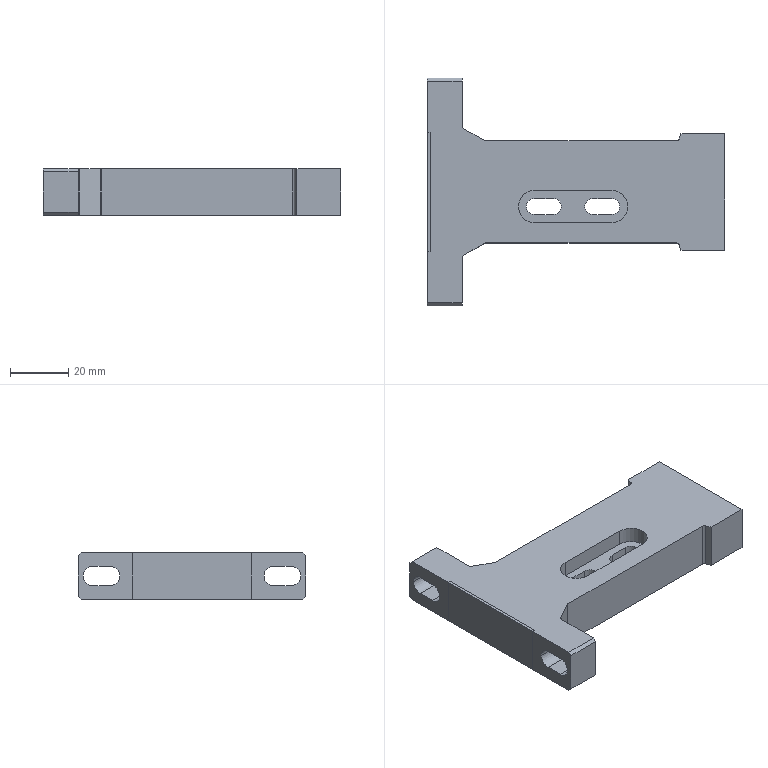NC program | NX | posted with a generic post | part box 102 x 78 x 16 mm
Lines 2875 to 2996 of 2996:
(FLOOR_WALL_1 , TOOL : D10JING)
N5748 T11 M6
N5750 G54
N5752 G17 G0 G90 X-14.997 Y-14. B0. C0. S9500 M3
N5754 G43 Z30. H11
N5756 Z0.
N5758 G94 G1 Z-1. F1250.
N5760 Y-13.
N5762 Y13.
N5764 X-9.998
N5766 Y-13.
N5768 X-4.998
N5770 Y13.
N5772 X0.001
N5774 Y-13.
N5776 X3.4
N5778 X5.001 Y-10.5
N5780 Y13.
N5782 X10.
N5784 Y-10.5
N5786 X11.5 Y-13.
N5788 X15.
N5790 Y13.
N5792 Y14.
N5794 Z0.
N5796 G0 Z30.
N5798 X15.5 Y-14.
N5800 Z0.
N5802 G1 Z-1.
N5804 Y-13.
N5806 Y13.
N5808 Y14.
N5810 Z0.
N5812 G0 Z30.
N5814 X-15.5
N5816 Z0.
N5818 G1 Z-1.
N5820 Y13.
N5822 Y-13.
N5824 Y-14.
N5826 Z0.
N5828 G0 Z30.
N5830 M5
(ZLEVEL_PROFILE_1_COPY_1_COPY_COPY_1 , TOOL : D6A45)
N5832 T07 M6
N5834 G54
N5836 G17 G0 G90 X27.868 Y-0.315 B0. C0. S9500 M3
N5838 G43 Z30. H7
N5840 Z-0.8
N5842 G94 G1 Z-1.8 F1000.
N5844 X27.48 Y-1.241
N5846 G3 X28. Y-1.541 R0.6
N5848 G1 X34.
N5850 G3 X35.541 Y0. R1.541
N5852 X34. Y1.541 R1.541
N5854 G1 X28.
N5856 G3 X26.459 Y0. R1.541
N5858 X28. Y-1.541 R1.541
N5860 X28.52 Y-1.241 R0.6
N5862 G1 X29.039 Y-0.341
N5864 Z-0.8
N5866 G0 Z30.
N5868 X-34.132 Y-0.315
N5870 Z-0.8
N5872 G1 Z-1.8
N5874 X-34.52 Y-1.241
N5876 G3 X-34. Y-1.541 R0.6
N5878 G1 X-28.
N5880 G3 X-26.459 Y0. R1.541
N5882 X-28. Y1.541 R1.541
N5884 G1 X-34.
N5886 G3 X-35.541 Y0. R1.541
N5888 X-34. Y-1.541 R1.541
N5890 X-33.48 Y-1.241 R0.6
N5892 G1 X-32.961 Y-0.341
N5894 Z-0.8
N5896 G0 Z30.
N5898 X-19.551 Y-10.801
N5900 Z-0.8
N5902 G1 Z-1.8
N5904 X-19.98 Y-10.059
N5906 G3 X-20.499 Y-9.759 R0.6
N5908 G1 X-38.001
N5910 G2 X-39.243 Y-9.244 R1.757
N5912 G1 X-40.244 Y-8.243
N5914 G2 X-40.759 Y-7.001 R1.757
N5916 G1 Y7.001
N5918 G2 X-40.244 Y8.243 R1.757
N5920 G1 X-39.243 Y9.244
N5922 G2 X-38.001 Y9.759 R1.757
N5924 G1 X-20.499
N5926 G2 X-18.915 Y8.759 R1.762
N5928 G1 X18.914
N5930 G2 X20.499 Y9.759 R1.763
N5932 G1 X38.001
N5934 G2 X39.243 Y9.244 R1.757
N5936 G1 X40.244 Y8.243
N5938 G2 X40.759 Y7.001 R1.757
N5940 G1 Y-7.001
N5942 G2 X40.244 Y-8.243 R1.757
N5944 G1 X39.243 Y-9.244
N5946 G2 X38.001 Y-9.759 R1.757
N5948 G1 X20.499
N5950 G2 X18.915 Y-8.759 R1.762
N5952 G1 X16.499
N5954 G2 X15.741 Y-8.001 R0.758
N5956 G1 Y-6.259
N5958 X-0.841
N5960 Y-8.001
N5962 G2 X-1.599 Y-8.759 R0.758
N5964 G1 X-18.914
N5966 G2 X-20.499 Y-9.759 R1.763
N5968 G3 X-21.018 Y-10.06 R0.6
N5970 G1 X-21.534 Y-10.959
N5972 Z-0.8
N5974 G0 Z30.
N5976 M5
N5978 M2